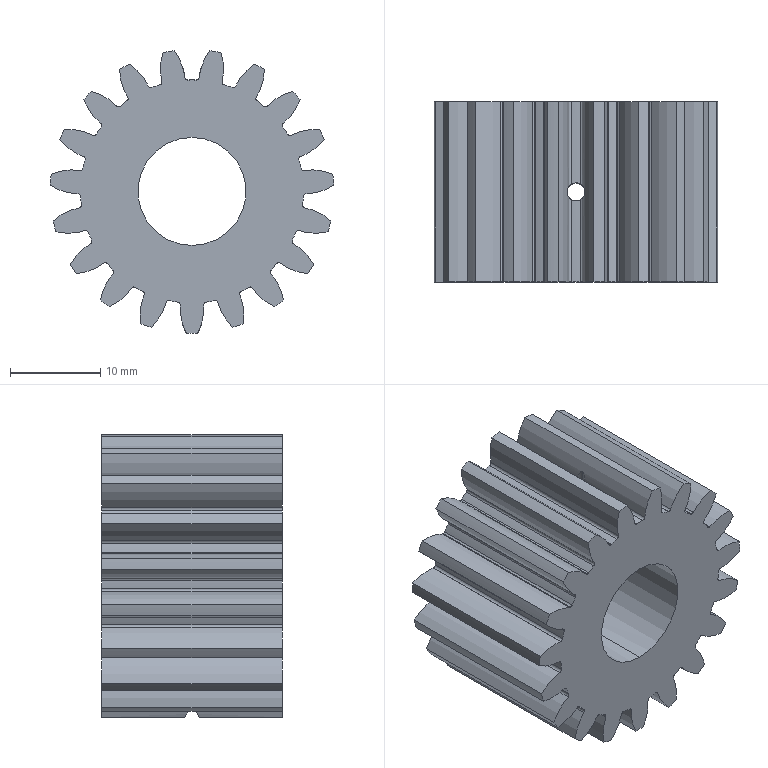Part | SolidWorks | features BaseBody 1 | 1 solid | 142 faces | box 31.47 x 20 x 31.374 mm | volume 10219 mm3 | cylinder 140 | plane 2 | commonest cylinder face diameters 0.6 x52 12.036 x40 31.5 x22 24.75 x20 2 x4 12 x2